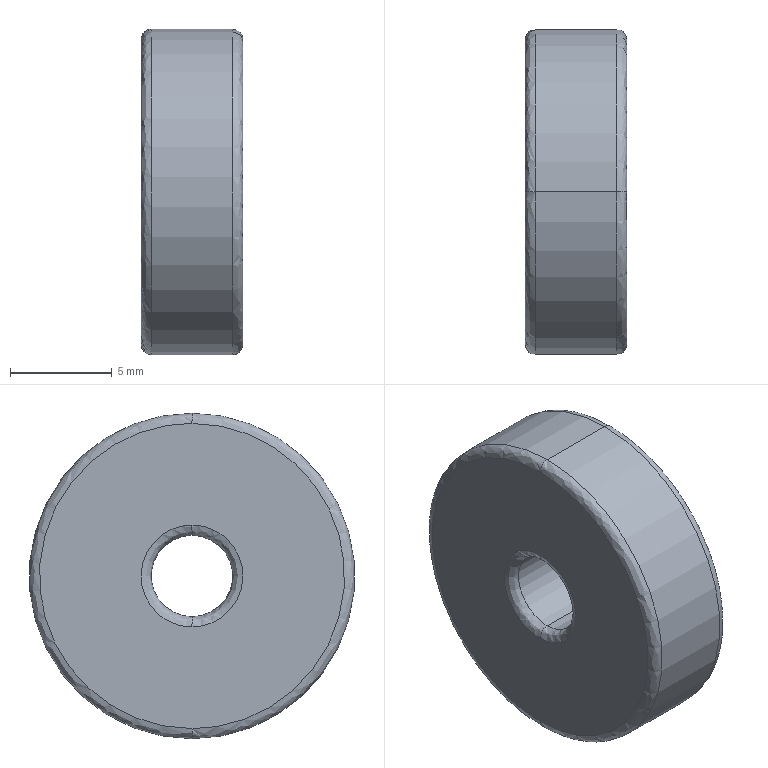Part | STEP file | Bearing SB634ZZ | 1 solid | 14 faces | box 5 x 16 x 16 mm | volume 935.765 mm3 | spline 8 | cylinder 4 | plane 2 | commonest cylinder face diameters 4 x2 16 x2